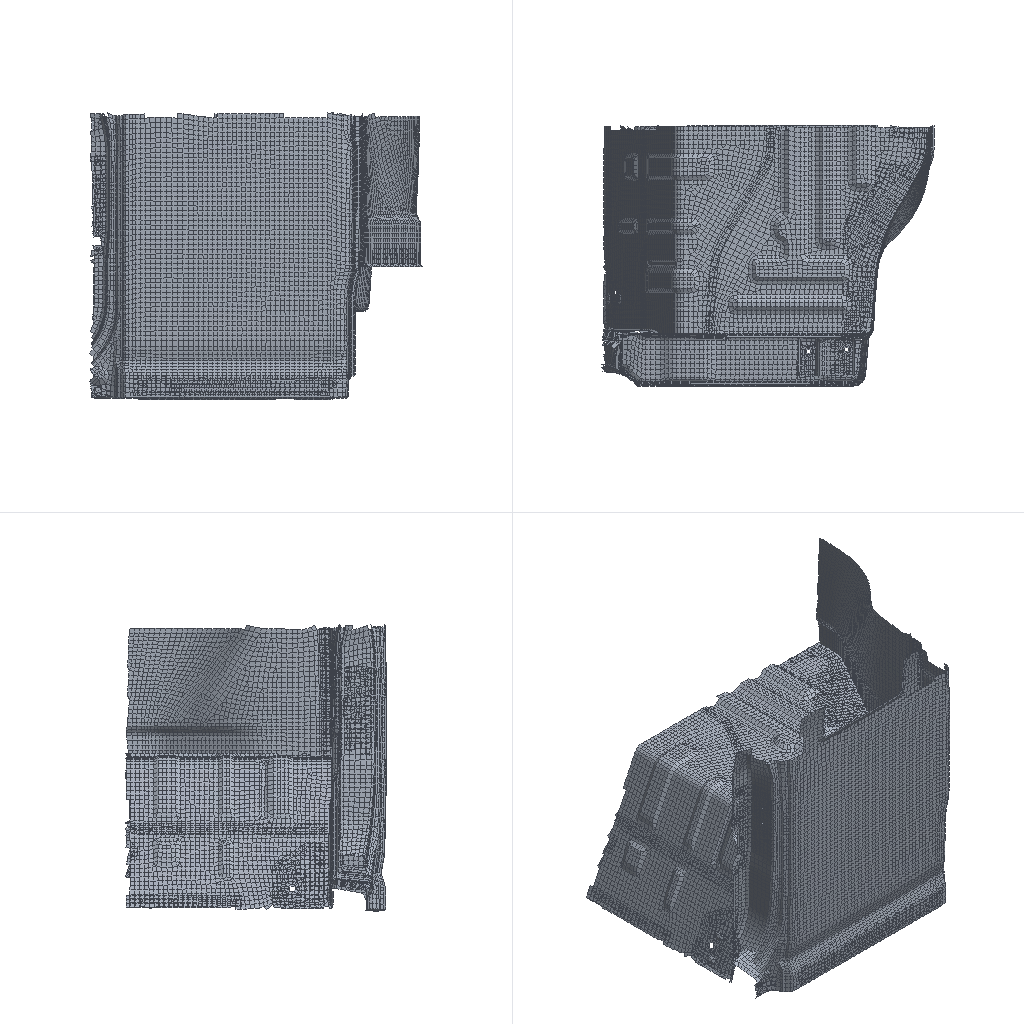Simulation study | nastran
Set-up summary:
category,name,step,type,value,unit,region
solver,nx_nastran
units,not stated in the deck,,not stated
analysis,deck,,static,static
analysis,solution,,SOL,101
load_step,SUBCASE 2,2,SUBCASE,SPC=2 LOAD=5
load_step,SUBCASE 3,3,SUBCASE,SPC=2 LOAD=4
load_step,SUBCASE 4,4,SUBCASE,SPC=2 LOAD=3
load_step,requested,,,3
mesh,nodes,,,23540
mesh,elements,,,21409
element_type,CHEXA,,solid,154
element_type,CQUAD4,,shell,20669
element_type,CTRIA3,,shell,586
load,load commands in deck,,count,3
bc,support commands in deck,,count,528
check,setup vs results,,match,"every grid point's frame and coordinates and every element id; grid points of CHEXA, CQUAD4, CTRIA3 elements"
Nastran input file, long lists of numbers shortened:
$$------------------------------------------------------------------------------$
$$                                                                              $
$$ NASTRAN Input Deck Generated by HyperMesh Version  :10.0buil                 $
$$ Generated using HyperMesh-Nastran Template Version : 10.0build60
$$                                                                              $
$$   Template:  general                                                         $
$$                                                                              $
$$------------------------------------------------------------------------------$
$$------------------------------------------------------------------------------$
$$                      Executive Control Cards                                 $
$$------------------------------------------------------------------------------$
SOL 101
CEND
$$------------------------------------------------------------------------------$
$$                      Case Control Cards                                      $
$$------------------------------------------------------------------------------$
  DISPLACEMENT = ALL
  ESE = ALL
$
$HMNAME LOADSTEP               2"fz"
SUBCASE       2
  LABEL=    fz
  SPC =        2
  LOAD =        5
$
$HMNAME LOADSTEP               3"fy"
SUBCASE       3
  LABEL=    fy
  SPC =        2
  LOAD =        4
$
$HMNAME LOADSTEP               4"fx"
SUBCASE       4
  LABEL=    fx
  SPC =        2
  LOAD =        3
$$------------------------------------------------------------------------------$
$$                      Bulk Data Cards                                         $
$$------------------------------------------------------------------------------$
BEGIN BULK
PARAM,POST,-1
$$
$$  GRID Data
$$
GRID       56565        765.8434-579.774628.3125
GRID       56566        765.8434-589.408628.3125
$ (23538 more lines like these left out)
$$
$$  SPOINT Data
$$
$$
$$------------------------------------------------------------------------------$
$$             Group Definitions                                                $
$$------------------------------------------------------------------------------$
$$
$$ RBE2 Elements - Multiple dependent nodes
$$
RBE2     102984684105773  123456 3577474 3577475 3577499 3577500 3577567+
+        3577568 3577569 3577570 3578590 3578591 3578620 3578621 3578683+
+        3578685 3578692 3578694 3611439 3611440 3611471 3611492 3611493+
+        3611494 3611495 3611496 3611497 3611498 3611499 3611500 3611501+
+        3611502 3611503 3611504 3611505 3611506 3611507 3611508 3611509+
+        3611510 3611511 3611512 3611514 3611515 3611516 3611517 3611519+
+        3611520 3611522 3611523 3611526 3611527 3611531 3611536 3611542+
+        3611551 3611555 3611560 3611565 3611817 3612136 3612977 3612978+
+        3613474 3613475 3614389 3614396 3614406 3615783 3615784 3615935+
+        3615936 3615944 3615945 3615951 3615952 3615953 3615960 3615961+
+        3615962 3616602 3616603 3616611 3616612 3616615 3616617 3616619+
+        3616621 3616622 3616623 3616624 3616625 3616626 3616627 3616628+
+        3616629 3616630 3616631 3616632 3616633 3616634 3616635 3616636+
+        3616637 3616638 3616639 3616640 3616641 3616642 3616643 3616648+
+        3617035 3617309 3617389 3617390 3617686 3617687 3617688 3617689+
+        3617857 3618277 3618278 3618419 3618420 3619309 3619310 3619646+
+        3619647 3619803 3619804 3619920 3619921 3619964 3619965 3620053+
+        3620054 3620057 3620058 3621354 3621355 3622988 3622989 3622995+
+        3622996 3623021 3623022 3623589 3623590 3623596 3623599 3623600+
+        3623925 3623926 3623935 3623936 3623938 3623939 3623941 3623942+
+        3623943 3623944 3623964 3623965 3623967 3623968 3623969 3623970+
+        3623973 3623974 3623975 3623976 3635506 3635507 3637069 3637089+
+        3637109 3637128 3637147 3637169 3637192 3637209 3637220 3637224+
+        3637234 3637239 3637247 3637253 3637262 3637267 3637276 3637281+
+        3637289 3637293 3637301 3637304 3637311 3639121 3639122 3639134+
+        3639135 3639136 3639140 3639141 3639142 3639443 3639444 3639770+
+        3639783 3639784 3639797 3639798 3639811 3639812 3639826 3639827+
+        3639842 3639844 3639856 3639858 3639871 3639873 3639885 3639886+
+        3639897 3639899 3639908 3639909 3639917 3639920 3639928 3639930+
+        3639940 3639941 3639954 3639956 3639971 3639972 3639986 3639988+
+        3640002 3640003 3640017 3703253 3703254 3703317 3703319 3703691+
+        3703692 3703756 3703757 3714444 3714445 3714484 3714485 3714486+
+        3714487 3714488 3714489 3715531 3722701 3722707 3722748 3722757+
+        3722824 3722835 3722836 3722847 3722848 3722858 3736764 3736767+
+        3736768 3736769 3736770 3736771 3736772 3736773 3736774 3736782+
+        3736783 3736784 3736785 3736786 3736787 3736788 3736789 3736790+
+        3738517 3738518 3738519 3738520 3738521 3738522 3738523 3738524+
+        3739112 3739113 3739114 3739115 3739116 3739117 3739118 3739119+
+        3739120 3739121 3739122 3739123 3739124 3739125 3739126 3739127+
+        3739128 3739129 3739130 3739131 3739132 3739133 3739134 3739135+
+        3739161 3739162 3739163 3739164 3739165 3739166 3739167 3739168+
+        3739169 3739170 3739171 3739172 3739173 3739174 3739175 3739176+
+        3739177 3739178 3739179 3739180 3739181 3739182 3739183 3739184+
+        3739185 3739186 3739195 3739196 3739197 3739198 3739199 3739200+
+        3739201 3739202 3739300 3739303 3739305 3739306 3739368 3739371+
+        3739372 3739390 3739391 3739392 3739393 3739394 3739395
$
$HMMOVE 84022702
$        1029846
$
$
$  RBE3 Elements
$
RBE3      326337         3755406  1234560.03889      123 37138720.025455+
+            123 37138710.370142     123 37138550.565513     123 3713854
RBE3      326338         3755407  1234560.623088     123 37138720.131026+
+            123 37138710.042722     123 37138550.203163     123 3713854
$ (2442 more lines like these left out)
$
$HMMOVE 57005012
$         326337THRU      326340  326342THRU      326349  326351THRU      326358
$         326360THRU      326367  326369THRU      326376  326378THRU      326385
$ (63 more lines like these left out)
CTRIA3    145590       9   58155   58153   58154
CTRIA3    145651       9   58249   58248   58239
$ (584 more lines like these left out)
$
$HMMOVE       14
$         145590  145651  145672  145684  145715  145720  145761THRU      145762
$         145769THRU      145770  145774  145778  145785  145804  148608  148800
$ (85 more lines like these left out)
CQUAD4    144410       9   56569   56613   56567   56568
CQUAD4    144411       9   56613   56614   56566   56567
$ (20667 more lines like these left out)
$
$HMMOVE       14
$         144410THRU      144415  144417THRU      144419  144422THRU      144424
$         144427THRU      144429  144433THRU      144435  144440THRU      144442
$ (542 more lines like these left out)
CHEXA     326341      10 3755406 3755409 3755408 3755407 3755410 3755413+
+        3755412 3755411
CHEXA     326350      10 3755415 3755416 3755417 3755418 3755419 3755420+
+        3755421 3755422
$ (304 more lines like these left out)
$
$HMMOVE 57005011
$         326341  326350  326359  326368  326377  326386  326395  326404  326413
$         326422  329221  329230  329239  329248  329257  329266  329383  329392
$ (106 more lines like these left out)
PSHELL         9       20.8            2               2
$
$HMNAME PROP                  10"120" 4
$HWCOLOR PROP                 10       3
PSHELL        10       21.2            2               2
$
$HMNAME PROP                  12"100" 4
$HWCOLOR PROP                 12       3
PSHELL        12       21.0            2               2
$
$HMNAME PROP                   5"150" 4
$HWCOLOR PROP                  5       3
PSHELL         5       21.5            2               2
$
$HMNAME PROP                  13"250" 4
$HWCOLOR PROP                 13       3
PSHELL        13       22.5            2               2
$
$HMNAME PROP                   7"200" 4
$HWCOLOR PROP                  7       3
PSHELL         7       22.0            2               2
$$
$$  PSOLID Data
$
$HMNAME PROP                  10"spot.1" 5
$HWCOLOR PROP                 10       3
PSOLID        10       2
$$
$$------------------------------------------------------------------------------$
$$                      Material Definition Cards                               $
$$------------------------------------------------------------------------------$
$$--------------------------------------------------------------
$$ HYPERMESH TAGS
$$--------------------------------------------------------------
$$BEGIN TAGS
$$END TAGS
$$
$$  MAT1 Data
$
$HMNAME MAT                    2"steel.1" "MAT1"
$HWCOLOR MAT                   2       3
MAT1           2210000.0        0.3     7.80E-09
$$
$$
$$
$$------------------------------------------------------------------------------$
$ (42 more lines like these left out)
SPC            2 3736000  1234560.0
SPC            2 3735999  1234560.0
SPC            2 3735581  1234560.0
SPC            2 3735574  1234560.0
$ (524 more lines like these left out)
$$
$$  FORCE Data
$$
FORCE          384105773       01.0     500.0   0.0     0.0
FORCE          484105773       01.0     0.0     500.0   0.0
FORCE          584105773       01.0     0.0     0.0     500.0
$HMASSEM       1       3 REAR_FLOOR
$HMASSEM_IDS    5100990084022690840226898402269651004810840226928402269351009911
$HMASSEM_IDS    8402269551001812510057108402269784022698
$HMASSEM      27       3 5600010.1
$HMASSEM_IDS          14
$HMASSEM 5400200       6 sidebody_R
$HMASSEM_IDS    54001220
$HMASSEM 5400100       7 sidebody_L
$HMASSEM_IDS    840226998402270154001210
$
ENDDATA
Results summary:
result,analysis,,,static
result,last_loadstep,,,3
result,primary field,,,displacements
result,max displacement,,,0.01057,model units